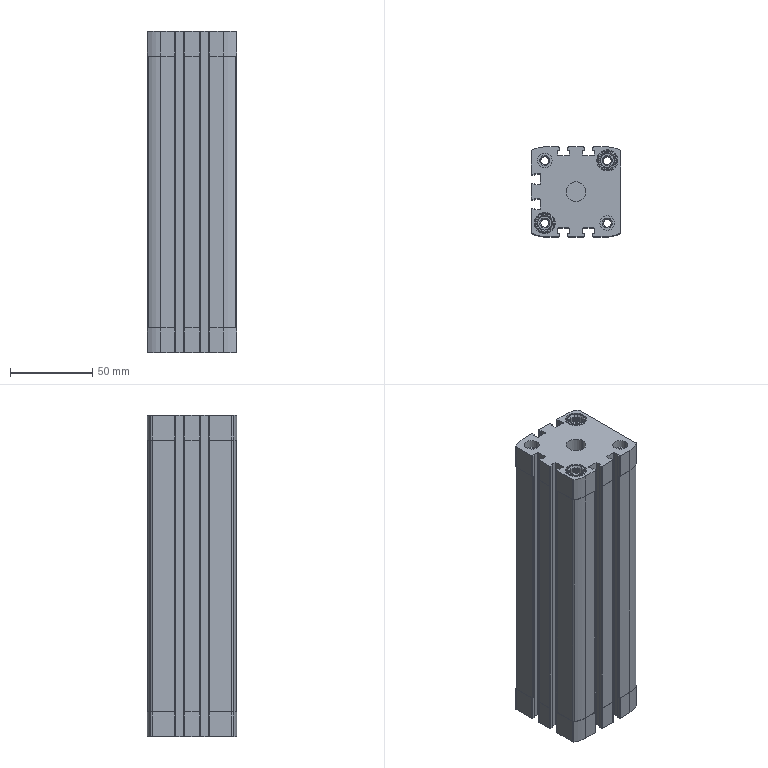Part | STEP file | HI_536288 ADN-150P-----(Z)_1-a_1_1 | 1 solid | 457 faces | box 54.5 x 54.5 x 195 mm | volume 304101 mm3 | plane 259 | cylinder 162 | cone 36 | commonest cylinder face diameters 0.8 x48 0.4 x24 4.917 x16 2 x12 29.6 x12 9 x10